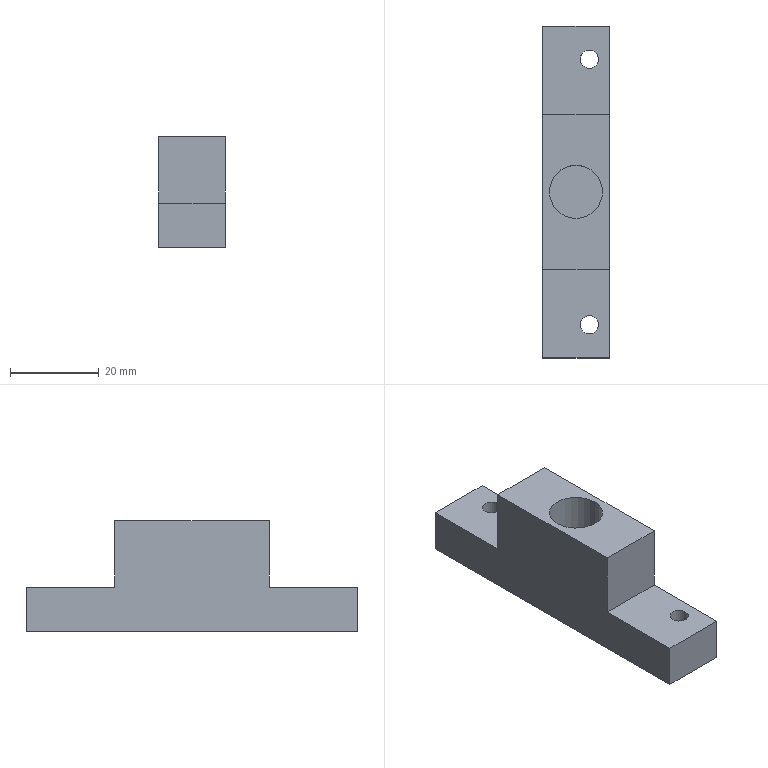Part | SolidWorks | features Cut 3, Extrusion 1 | 1 solid | 17 faces | box 15 x 75 x 25 mm | volume 16595 mm3 | plane 11 | cylinder 6 | commonest cylinder face diameters 4.134 x4 12 x2
STEP:
#1=CARTESIAN_POINT('',(-35.5,0.,5.));
#2=VERTEX_POINT('',#1);
#3=CARTESIAN_POINT('',(-23.5,0.,5.));
#4=VERTEX_POINT('',#3);
#5=CARTESIAN_POINT('',(-29.5,0.,5.));
#6=DIRECTION('',(0.,0.,1.));
#7=DIRECTION('',(1.,0.,0.));
#8=AXIS2_PLACEMENT_3D('',#5,#6,#7);
#9=CIRCLE('',#8,6.);
#10=EDGE_CURVE('',#2,#4,#9,.T.);
#11=ORIENTED_EDGE('',*,*,#10,.F.);
#12=CARTESIAN_POINT('',(-35.5,0.,25.));
#13=VERTEX_POINT('',#12);
#14=CARTESIAN_POINT('',(-35.5,0.,5.));
#15=DIRECTION('',(0.,0.,1.));
#16=VECTOR('',#15,1000.);
#17=LINE('',#14,#16);
#18=EDGE_CURVE('',#2,#13,#17,.T.);
#19=ORIENTED_EDGE('',*,*,#18,.T.);
#20=CARTESIAN_POINT('',(-23.5,0.,25.));
#21=VERTEX_POINT('',#20);
#22=CARTESIAN_POINT('',(-29.5,0.,25.));
#23=DIRECTION('',(0.,0.,1.));
#24=DIRECTION('',(1.,0.,0.));
#25=AXIS2_PLACEMENT_3D('',#22,#23,#24);
#26=CIRCLE('',#25,6.);
#27=EDGE_CURVE('',#13,#21,#26,.T.);
#28=ORIENTED_EDGE('',*,*,#27,.T.);
#29=CARTESIAN_POINT('',(-23.5,0.,5.));
#30=DIRECTION('',(0.,0.,1.));
#31=VECTOR('',#30,1000.);
#32=LINE('',#29,#31);
#33=EDGE_CURVE('',#4,#21,#32,.T.);
#34=ORIENTED_EDGE('',*,*,#33,.F.);
#35=EDGE_LOOP('',(#11,#19,#28,#34));
#36=FACE_OUTER_BOUND('',#35,.T.);
#37=CARTESIAN_POINT('',(-29.5,0.,5.));
#38=DIRECTION('',(0.,0.,1.));
#39=DIRECTION('',(1.,0.,0.));
#40=AXIS2_PLACEMENT_3D('',#37,#38,#39);
#41=CYLINDRICAL_SURFACE('',#40,6.);
#42=ADVANCED_FACE('',(#36),#41,.F.);
#43=CARTESIAN_POINT('',(-28.567,30.,0.));
#44=VERTEX_POINT('',#43);
#45=CARTESIAN_POINT('',(-24.433,30.,0.));
#46=VERTEX_POINT('',#45);
#47=CARTESIAN_POINT('',(-26.5,30.,0.));
#48=DIRECTION('',(0.,0.,1.));
#49=DIRECTION('',(1.,0.,0.));
#50=AXIS2_PLACEMENT_3D('',#47,#48,#49);
#51=CIRCLE('',#50,2.067);
#52=EDGE_CURVE('',#44,#46,#51,.T.);
#53=ORIENTED_EDGE('',*,*,#52,.F.);
#54=CARTESIAN_POINT('',(-28.567,30.,10.));
#55=VERTEX_POINT('',#54);
#56=CARTESIAN_POINT('',(-28.567,30.,0.));
#57=DIRECTION('',(0.,0.,1.));
#58=VECTOR('',#57,1000.);
#59=LINE('',#56,#58);
#60=EDGE_CURVE('',#44,#55,#59,.T.);
#61=ORIENTED_EDGE('',*,*,#60,.T.);
#62=CARTESIAN_POINT('',(-24.433,30.,10.));
#63=VERTEX_POINT('',#62);
#64=CARTESIAN_POINT('',(-26.5,30.,10.));
#65=DIRECTION('',(0.,0.,1.));
#66=DIRECTION('',(-1.,0.,0.));
#67=AXIS2_PLACEMENT_3D('',#64,#65,#66);
#68=CIRCLE('',#67,2.067);
#69=EDGE_CURVE('',#55,#63,#68,.T.);
#70=ORIENTED_EDGE('',*,*,#69,.T.);
#71=CARTESIAN_POINT('',(-24.433,30.,0.));
#72=DIRECTION('',(0.,0.,1.));
#73=VECTOR('',#72,1000.);
#74=LINE('',#71,#73);
#75=EDGE_CURVE('',#46,#63,#74,.T.);
#76=ORIENTED_EDGE('',*,*,#75,.F.);
#77=EDGE_LOOP('',(#53,#61,#70,#76));
#78=FACE_OUTER_BOUND('',#77,.T.);
#79=CARTESIAN_POINT('',(-26.5,30.,0.));
#80=DIRECTION('',(0.,0.,1.));
#81=DIRECTION('',(1.,0.,0.));
#82=AXIS2_PLACEMENT_3D('',#79,#80,#81);
#83=CYLINDRICAL_SURFACE('',#82,2.067);
#84=ADVANCED_FACE('',(#78),#83,.F.);
#85=CARTESIAN_POINT('',(-28.567,-30.,0.));
#86=VERTEX_POINT('',#85);
#87=CARTESIAN_POINT('',(-24.433,-30.,0.));
#88=VERTEX_POINT('',#87);
#89=CARTESIAN_POINT('',(-26.5,-30.,0.));
#90=DIRECTION('',(0.,0.,1.));
#91=DIRECTION('',(1.,0.,0.));
#92=AXIS2_PLACEMENT_3D('',#89,#90,#91);
#93=CIRCLE('',#92,2.067);
#94=EDGE_CURVE('',#86,#88,#93,.T.);
#95=ORIENTED_EDGE('',*,*,#94,.F.);
#96=CARTESIAN_POINT('',(-28.567,-30.,10.));
#97=VERTEX_POINT('',#96);
#98=CARTESIAN_POINT('',(-28.567,-30.,0.));
#99=DIRECTION('',(0.,0.,1.));
#100=VECTOR('',#99,1000.);
#101=LINE('',#98,#100);
#102=EDGE_CURVE('',#86,#97,#101,.T.);
#103=ORIENTED_EDGE('',*,*,#102,.T.);
#104=CARTESIAN_POINT('',(-24.433,-30.,10.));
#105=VERTEX_POINT('',#104);
#106=CARTESIAN_POINT('',(-26.5,-30.,10.));
#107=DIRECTION('',(0.,0.,-1.));
#108=DIRECTION('',(1.,0.,0.));
#109=AXIS2_PLACEMENT_3D('',#106,#107,#108);
#110=CIRCLE('',#109,2.067);
#111=EDGE_CURVE('',#105,#97,#110,.T.);
#112=ORIENTED_EDGE('',*,*,#111,.F.);
#113=CARTESIAN_POINT('',(-24.433,-30.,0.));
#114=DIRECTION('',(0.,0.,1.));
#115=VECTOR('',#114,1000.);
#116=LINE('',#113,#115);
#117=EDGE_CURVE('',#88,#105,#116,.T.);
#118=ORIENTED_EDGE('',*,*,#117,.F.);
#119=EDGE_LOOP('',(#95,#103,#112,#118));
#120=FACE_OUTER_BOUND('',#119,.T.);
#121=CARTESIAN_POINT('',(-26.5,-30.,0.));
#122=DIRECTION('',(0.,0.,1.));
#123=DIRECTION('',(1.,0.,0.));
#124=AXIS2_PLACEMENT_3D('',#121,#122,#123);
#125=CYLINDRICAL_SURFACE('',#124,2.067);
#126=ADVANCED_FACE('',(#120),#125,.F.);
#127=CARTESIAN_POINT('',(-37.,-37.5,10.));
#128=VERTEX_POINT('',#127);
#129=CARTESIAN_POINT('',(-22.,-37.5,10.));
#130=VERTEX_POINT('',#129);
#131=CARTESIAN_POINT('',(-37.,-37.5,10.));
#132=DIRECTION('',(1.,0.,0.));
#133=VECTOR('',#132,1000.);
#134=LINE('',#131,#133);
#135=EDGE_CURVE('',#128,#130,#134,.T.);
#136=ORIENTED_EDGE('',*,*,#135,.F.);
#137=CARTESIAN_POINT('',(-37.,-37.5,0.));
#138=VERTEX_POINT('',#137);
#139=CARTESIAN_POINT('',(-37.,-37.5,25.));
#140=DIRECTION('',(0.,0.,-1.));
#141=VECTOR('',#140,1000.);
#142=LINE('',#139,#141);
#143=EDGE_CURVE('',#128,#138,#142,.T.);
#144=ORIENTED_EDGE('',*,*,#143,.T.);
#145=CARTESIAN_POINT('',(-22.,-37.5,0.));
#146=VERTEX_POINT('',#145);
#147=CARTESIAN_POINT('',(-22.,-37.5,0.));
#148=DIRECTION('',(1.,0.,0.));
#149=VECTOR('',#148,1000.);
#150=LINE('',#147,#149);
#151=EDGE_CURVE('',#138,#146,#150,.T.);
#152=ORIENTED_EDGE('',*,*,#151,.T.);
#153=CARTESIAN_POINT('',(-22.,-37.5,25.));
#154=DIRECTION('',(0.,0.,-1.));
#155=VECTOR('',#154,1000.);
#156=LINE('',#153,#155);
#157=EDGE_CURVE('',#130,#146,#156,.T.);
#158=ORIENTED_EDGE('',*,*,#157,.F.);
#159=EDGE_LOOP('',(#136,#144,#152,#158));
#160=FACE_OUTER_BOUND('',#159,.T.);
#161=CARTESIAN_POINT('',(-22.,-37.5,25.));
#162=DIRECTION('',(0.,1.,0.));
#163=DIRECTION('',(0.,0.,1.));
#164=AXIS2_PLACEMENT_3D('',#161,#162,#163);
#165=PLANE('',#164);
#166=ADVANCED_FACE('',(#160),#165,.F.);
#167=ORIENTED_EDGE('',*,*,#102,.F.);
#168=CARTESIAN_POINT('',(-26.5,-30.,0.));
#169=DIRECTION('',(0.,0.,1.));
#170=DIRECTION('',(1.,0.,0.));
#171=AXIS2_PLACEMENT_3D('',#168,#169,#170);
#172=CIRCLE('',#171,2.067);
#173=EDGE_CURVE('',#88,#86,#172,.T.);
#174=ORIENTED_EDGE('',*,*,#173,.F.);
#175=ORIENTED_EDGE('',*,*,#117,.T.);
#176=CARTESIAN_POINT('',(-26.5,-30.,10.));
#177=DIRECTION('',(0.,0.,-1.));
#178=DIRECTION('',(1.,0.,0.));
#179=AXIS2_PLACEMENT_3D('',#176,#177,#178);
#180=CIRCLE('',#179,2.067);
#181=EDGE_CURVE('',#97,#105,#180,.T.);
#182=ORIENTED_EDGE('',*,*,#181,.F.);
#183=EDGE_LOOP('',(#167,#174,#175,#182));
#184=FACE_OUTER_BOUND('',#183,.T.);
#185=CARTESIAN_POINT('',(-26.5,-30.,0.));
#186=DIRECTION('',(0.,0.,1.));
#187=DIRECTION('',(1.,0.,0.));
#188=AXIS2_PLACEMENT_3D('',#185,#186,#187);
#189=CYLINDRICAL_SURFACE('',#188,2.067);
#190=ADVANCED_FACE('',(#184),#189,.F.);
#191=CARTESIAN_POINT('',(-37.,37.5,10.));
#192=VERTEX_POINT('',#191);
#193=CARTESIAN_POINT('',(-37.,37.5,0.));
#194=VERTEX_POINT('',#193);
#195=CARTESIAN_POINT('',(-37.,37.5,25.));
#196=DIRECTION('',(0.,0.,-1.));
#197=VECTOR('',#196,1000.);
#198=LINE('',#195,#197);
#199=EDGE_CURVE('',#192,#194,#198,.T.);
#200=ORIENTED_EDGE('',*,*,#199,.F.);
#201=CARTESIAN_POINT('',(-22.,37.5,10.));
#202=VERTEX_POINT('',#201);
#203=CARTESIAN_POINT('',(-37.,37.5,10.));
#204=DIRECTION('',(-1.,0.,0.));
#205=VECTOR('',#204,1000.);
#206=LINE('',#203,#205);
#207=EDGE_CURVE('',#202,#192,#206,.T.);
#208=ORIENTED_EDGE('',*,*,#207,.F.);
#209=CARTESIAN_POINT('',(-22.,37.5,0.));
#210=VERTEX_POINT('',#209);
#211=CARTESIAN_POINT('',(-22.,37.5,25.));
#212=DIRECTION('',(0.,0.,-1.));
#213=VECTOR('',#212,1000.);
#214=LINE('',#211,#213);
#215=EDGE_CURVE('',#202,#210,#214,.T.);
#216=ORIENTED_EDGE('',*,*,#215,.T.);
#217=CARTESIAN_POINT('',(-37.,37.5,0.));
#218=DIRECTION('',(-1.,0.,0.));
#219=VECTOR('',#218,1000.);
#220=LINE('',#217,#219);
#221=EDGE_CURVE('',#210,#194,#220,.T.);
#222=ORIENTED_EDGE('',*,*,#221,.T.);
#223=EDGE_LOOP('',(#200,#208,#216,#222));
#224=FACE_OUTER_BOUND('',#223,.T.);
#225=CARTESIAN_POINT('',(-37.,37.5,25.));
#226=DIRECTION('',(0.,-1.,0.));
#227=DIRECTION('',(0.,0.,-1.));
#228=AXIS2_PLACEMENT_3D('',#225,#226,#227);
#229=PLANE('',#228);
#230=ADVANCED_FACE('',(#224),#229,.F.);
#231=CARTESIAN_POINT('',(-37.,17.5,25.));
#232=VERTEX_POINT('',#231);
#233=CARTESIAN_POINT('',(-37.,-17.5,25.));
#234=VERTEX_POINT('',#233);
#235=CARTESIAN_POINT('',(-37.,-37.5,25.));
#236=DIRECTION('',(0.,-1.,0.));
#237=VECTOR('',#236,1000.);
#238=LINE('',#235,#237);
#239=EDGE_CURVE('',#232,#234,#238,.T.);
#240=ORIENTED_EDGE('',*,*,#239,.F.);
#241=CARTESIAN_POINT('',(-37.,17.5,10.));
#242=VERTEX_POINT('',#241);
#243=CARTESIAN_POINT('',(-37.,17.5,10.));
#244=DIRECTION('',(0.,0.,1.));
#245=VECTOR('',#244,1000.);
#246=LINE('',#243,#245);
#247=EDGE_CURVE('',#242,#232,#246,.T.);
#248=ORIENTED_EDGE('',*,*,#247,.F.);
#249=CARTESIAN_POINT('',(-37.,17.5,10.));
#250=DIRECTION('',(0.,-1.,0.));
#251=VECTOR('',#250,1000.);
#252=LINE('',#249,#251);
#253=EDGE_CURVE('',#192,#242,#252,.T.);
#254=ORIENTED_EDGE('',*,*,#253,.F.);
#255=ORIENTED_EDGE('',*,*,#199,.T.);
#256=CARTESIAN_POINT('',(-37.,-37.5,0.));
#257=DIRECTION('',(0.,-1.,0.));
#258=VECTOR('',#257,1000.);
#259=LINE('',#256,#258);
#260=EDGE_CURVE('',#194,#138,#259,.T.);
#261=ORIENTED_EDGE('',*,*,#260,.T.);
#262=ORIENTED_EDGE('',*,*,#143,.F.);
#263=CARTESIAN_POINT('',(-37.,-17.5,10.));
#264=VERTEX_POINT('',#263);
#265=CARTESIAN_POINT('',(-37.,-17.5,10.));
#266=DIRECTION('',(0.,-1.,0.));
#267=VECTOR('',#266,1000.);
#268=LINE('',#265,#267);
#269=EDGE_CURVE('',#264,#128,#268,.T.);
#270=ORIENTED_EDGE('',*,*,#269,.F.);
#271=CARTESIAN_POINT('',(-37.,-17.5,10.));
#272=DIRECTION('',(0.,0.,1.));
#273=VECTOR('',#272,1000.);
#274=LINE('',#271,#273);
#275=EDGE_CURVE('',#264,#234,#274,.T.);
#276=ORIENTED_EDGE('',*,*,#275,.T.);
#277=EDGE_LOOP('',(#240,#248,#254,#255,#261,#262,#270,#276));
#278=FACE_OUTER_BOUND('',#277,.T.);
#279=CARTESIAN_POINT('',(-37.,-37.5,25.));
#280=DIRECTION('',(1.,0.,0.));
#281=DIRECTION('',(0.,0.,-1.));
#282=AXIS2_PLACEMENT_3D('',#279,#280,#281);
#283=PLANE('',#282);
#284=ADVANCED_FACE('',(#278),#283,.F.);
#285=CARTESIAN_POINT('',(-22.,17.5,10.));
#286=VERTEX_POINT('',#285);
#287=CARTESIAN_POINT('',(-22.,37.5,10.));
#288=DIRECTION('',(0.,1.,0.));
#289=VECTOR('',#288,1000.);
#290=LINE('',#287,#289);
#291=EDGE_CURVE('',#286,#202,#290,.T.);
#292=ORIENTED_EDGE('',*,*,#291,.F.);
#293=CARTESIAN_POINT('',(-22.,17.5,25.));
#294=VERTEX_POINT('',#293);
#295=CARTESIAN_POINT('',(-22.,17.5,10.));
#296=DIRECTION('',(0.,0.,1.));
#297=VECTOR('',#296,1000.);
#298=LINE('',#295,#297);
#299=EDGE_CURVE('',#286,#294,#298,.T.);
#300=ORIENTED_EDGE('',*,*,#299,.T.);
#301=CARTESIAN_POINT('',(-22.,-17.5,25.));
#302=VERTEX_POINT('',#301);
#303=CARTESIAN_POINT('',(-22.,37.5,25.));
#304=DIRECTION('',(0.,1.,0.));
#305=VECTOR('',#304,1000.);
#306=LINE('',#303,#305);
#307=EDGE_CURVE('',#302,#294,#306,.T.);
#308=ORIENTED_EDGE('',*,*,#307,.F.);
#309=CARTESIAN_POINT('',(-22.,-17.5,10.));
#310=VERTEX_POINT('',#309);
#311=CARTESIAN_POINT('',(-22.,-17.5,10.));
#312=DIRECTION('',(0.,0.,1.));
#313=VECTOR('',#312,1000.);
#314=LINE('',#311,#313);
#315=EDGE_CURVE('',#310,#302,#314,.T.);
#316=ORIENTED_EDGE('',*,*,#315,.F.);
#317=CARTESIAN_POINT('',(-22.,-37.5,10.));
#318=DIRECTION('',(0.,1.,0.));
#319=VECTOR('',#318,1000.);
#320=LINE('',#317,#319);
#321=EDGE_CURVE('',#130,#310,#320,.T.);
#322=ORIENTED_EDGE('',*,*,#321,.F.);
#323=ORIENTED_EDGE('',*,*,#157,.T.);
#324=CARTESIAN_POINT('',(-22.,37.5,0.));
#325=DIRECTION('',(0.,1.,0.));
#326=VECTOR('',#325,1000.);
#327=LINE('',#324,#326);
#328=EDGE_CURVE('',#146,#210,#327,.T.);
#329=ORIENTED_EDGE('',*,*,#328,.T.);
#330=ORIENTED_EDGE('',*,*,#215,.F.);
#331=EDGE_LOOP('',(#292,#300,#308,#316,#322,#323,#329,#330));
#332=FACE_OUTER_BOUND('',#331,.T.);
#333=CARTESIAN_POINT('',(-22.,37.5,25.));
#334=DIRECTION('',(-1.,0.,0.));
#335=DIRECTION('',(0.,-1.,0.));
#336=AXIS2_PLACEMENT_3D('',#333,#334,#335);
#337=PLANE('',#336);
#338=ADVANCED_FACE('',(#332),#337,.F.);
#339=CARTESIAN_POINT('',(-29.5,0.,25.));
#340=DIRECTION('',(0.,0.,1.));
#341=DIRECTION('',(1.,0.,0.));
#342=AXIS2_PLACEMENT_3D('',#339,#340,#341);
#343=CIRCLE('',#342,6.);
#344=EDGE_CURVE('',#21,#13,#343,.T.);
#345=ORIENTED_EDGE('',*,*,#344,.F.);
#346=ORIENTED_EDGE('',*,*,#27,.F.);
#347=EDGE_LOOP('',(#345,#346));
#348=FACE_BOUND('',#347,.T.);
#349=ORIENTED_EDGE('',*,*,#307,.T.);
#350=CARTESIAN_POINT('',(-22.,17.5,25.));
#351=DIRECTION('',(1.,0.,0.));
#352=VECTOR('',#351,1000.);
#353=LINE('',#350,#352);
#354=EDGE_CURVE('',#232,#294,#353,.T.);
#355=ORIENTED_EDGE('',*,*,#354,.F.);
#356=ORIENTED_EDGE('',*,*,#239,.T.);
#357=CARTESIAN_POINT('',(-22.,-17.5,25.));
#358=DIRECTION('',(-1.,0.,0.));
#359=VECTOR('',#358,1000.);
#360=LINE('',#357,#359);
#361=EDGE_CURVE('',#302,#234,#360,.T.);
#362=ORIENTED_EDGE('',*,*,#361,.F.);
#363=EDGE_LOOP('',(#349,#355,#356,#362));
#364=FACE_OUTER_BOUND('',#363,.T.);
#365=CARTESIAN_POINT('',(0.,0.,25.));
#366=DIRECTION('',(0.,0.,-1.));
#367=DIRECTION('',(-1.,0.,0.));
#368=AXIS2_PLACEMENT_3D('',#365,#366,#367);
#369=PLANE('',#368);
#370=ADVANCED_FACE('',(#348,#364),#369,.F.);
#371=CARTESIAN_POINT('',(-26.5,30.,0.));
#372=DIRECTION('',(0.,0.,1.));
#373=DIRECTION('',(1.,0.,0.));
#374=AXIS2_PLACEMENT_3D('',#371,#372,#373);
#375=CIRCLE('',#374,2.067);
#376=EDGE_CURVE('',#46,#44,#375,.T.);
#377=ORIENTED_EDGE('',*,*,#376,.T.);
#378=ORIENTED_EDGE('',*,*,#52,.T.);
#379=EDGE_LOOP('',(#377,#378));
#380=FACE_BOUND('',#379,.T.);
#381=ORIENTED_EDGE('',*,*,#173,.T.);
#382=ORIENTED_EDGE('',*,*,#94,.T.);
#383=EDGE_LOOP('',(#381,#382));
#384=FACE_BOUND('',#383,.T.);
#385=ORIENTED_EDGE('',*,*,#221,.F.);
#386=ORIENTED_EDGE('',*,*,#328,.F.);
#387=ORIENTED_EDGE('',*,*,#151,.F.);
#388=ORIENTED_EDGE('',*,*,#260,.F.);
#389=EDGE_LOOP('',(#385,#386,#387,#388));
#390=FACE_OUTER_BOUND('',#389,.T.);
#391=CARTESIAN_POINT('',(0.,0.,0.));
#392=DIRECTION('',(0.,0.,-1.));
#393=DIRECTION('',(-1.,0.,0.));
#394=AXIS2_PLACEMENT_3D('',#391,#392,#393);
#395=PLANE('',#394);
#396=ADVANCED_FACE('',(#380,#384,#390),#395,.T.);
#397=ORIENTED_EDGE('',*,*,#60,.F.);
#398=ORIENTED_EDGE('',*,*,#376,.F.);
#399=ORIENTED_EDGE('',*,*,#75,.T.);
#400=CARTESIAN_POINT('',(-26.5,30.,10.));
#401=DIRECTION('',(0.,0.,1.));
#402=DIRECTION('',(-1.,0.,0.));
#403=AXIS2_PLACEMENT_3D('',#400,#401,#402);
#404=CIRCLE('',#403,2.067);
#405=EDGE_CURVE('',#63,#55,#404,.T.);
#406=ORIENTED_EDGE('',*,*,#405,.T.);
#407=EDGE_LOOP('',(#397,#398,#399,#406));
#408=FACE_OUTER_BOUND('',#407,.T.);
#409=CARTESIAN_POINT('',(-26.5,30.,0.));
#410=DIRECTION('',(0.,0.,1.));
#411=DIRECTION('',(1.,0.,0.));
#412=AXIS2_PLACEMENT_3D('',#409,#410,#411);
#413=CYLINDRICAL_SURFACE('',#412,2.067);
#414=ADVANCED_FACE('',(#408),#413,.F.);
#415=ORIENTED_EDGE('',*,*,#253,.T.);
#416=CARTESIAN_POINT('',(-22.,17.5,10.));
#417=DIRECTION('',(1.,0.,0.));
#418=VECTOR('',#417,1000.);
#419=LINE('',#416,#418);
#420=EDGE_CURVE('',#242,#286,#419,.T.);
#421=ORIENTED_EDGE('',*,*,#420,.T.);
#422=ORIENTED_EDGE('',*,*,#291,.T.);
#423=ORIENTED_EDGE('',*,*,#207,.T.);
#424=EDGE_LOOP('',(#415,#421,#422,#423));
#425=FACE_OUTER_BOUND('',#424,.T.);
#426=ORIENTED_EDGE('',*,*,#405,.F.);
#427=ORIENTED_EDGE('',*,*,#69,.F.);
#428=EDGE_LOOP('',(#426,#427));
#429=FACE_BOUND('',#428,.T.);
#430=CARTESIAN_POINT('',(0.,0.,10.));
#431=DIRECTION('',(0.,0.,-1.));
#432=DIRECTION('',(-1.,0.,0.));
#433=AXIS2_PLACEMENT_3D('',#430,#431,#432);
#434=PLANE('',#433);
#435=ADVANCED_FACE('',(#425,#429),#434,.F.);
#436=ORIENTED_EDGE('',*,*,#354,.T.);
#437=ORIENTED_EDGE('',*,*,#299,.F.);
#438=ORIENTED_EDGE('',*,*,#420,.F.);
#439=ORIENTED_EDGE('',*,*,#247,.T.);
#440=EDGE_LOOP('',(#436,#437,#438,#439));
#441=FACE_OUTER_BOUND('',#440,.T.);
#442=CARTESIAN_POINT('',(-22.,17.5,10.));
#443=DIRECTION('',(0.,-1.,0.));
#444=DIRECTION('',(0.,0.,-1.));
#445=AXIS2_PLACEMENT_3D('',#442,#443,#444);
#446=PLANE('',#445);
#447=ADVANCED_FACE('',(#441),#446,.F.);
#448=ORIENTED_EDGE('',*,*,#321,.T.);
#449=CARTESIAN_POINT('',(-22.,-17.5,10.));
#450=DIRECTION('',(-1.,0.,0.));
#451=VECTOR('',#450,1000.);
#452=LINE('',#449,#451);
#453=EDGE_CURVE('',#310,#264,#452,.T.);
#454=ORIENTED_EDGE('',*,*,#453,.T.);
#455=ORIENTED_EDGE('',*,*,#269,.T.);
#456=ORIENTED_EDGE('',*,*,#135,.T.);
#457=EDGE_LOOP('',(#448,#454,#455,#456));
#458=FACE_OUTER_BOUND('',#457,.T.);
#459=ORIENTED_EDGE('',*,*,#111,.T.);
#460=ORIENTED_EDGE('',*,*,#181,.T.);
#461=EDGE_LOOP('',(#459,#460));
#462=FACE_BOUND('',#461,.T.);
#463=CARTESIAN_POINT('',(0.,0.,10.));
#464=DIRECTION('',(0.,0.,1.));
#465=DIRECTION('',(1.,0.,0.));
#466=AXIS2_PLACEMENT_3D('',#463,#464,#465);
#467=PLANE('',#466);
#468=ADVANCED_FACE('',(#458,#462),#467,.T.);
#469=ORIENTED_EDGE('',*,*,#361,.T.);
#470=ORIENTED_EDGE('',*,*,#275,.F.);
#471=ORIENTED_EDGE('',*,*,#453,.F.);
#472=ORIENTED_EDGE('',*,*,#315,.T.);
#473=EDGE_LOOP('',(#469,#470,#471,#472));
#474=FACE_OUTER_BOUND('',#473,.T.);
#475=CARTESIAN_POINT('',(-22.,-17.5,10.));
#476=DIRECTION('',(0.,1.,0.));
#477=DIRECTION('',(0.,0.,1.));
#478=AXIS2_PLACEMENT_3D('',#475,#476,#477);
#479=PLANE('',#478);
#480=ADVANCED_FACE('',(#474),#479,.F.);
#481=ORIENTED_EDGE('',*,*,#18,.F.);
#482=CARTESIAN_POINT('',(-29.5,0.,5.));
#483=DIRECTION('',(0.,0.,1.));
#484=DIRECTION('',(1.,0.,0.));
#485=AXIS2_PLACEMENT_3D('',#482,#483,#484);
#486=CIRCLE('',#485,6.);
#487=EDGE_CURVE('',#4,#2,#486,.T.);
#488=ORIENTED_EDGE('',*,*,#487,.F.);
#489=ORIENTED_EDGE('',*,*,#33,.T.);
#490=ORIENTED_EDGE('',*,*,#344,.T.);
#491=EDGE_LOOP('',(#481,#488,#489,#490));
#492=FACE_OUTER_BOUND('',#491,.T.);
#493=CARTESIAN_POINT('',(-29.5,0.,5.));
#494=DIRECTION('',(0.,0.,1.));
#495=DIRECTION('',(1.,0.,0.));
#496=AXIS2_PLACEMENT_3D('',#493,#494,#495);
#497=CYLINDRICAL_SURFACE('',#496,6.);
#498=ADVANCED_FACE('',(#492),#497,.F.);
#499=ORIENTED_EDGE('',*,*,#487,.T.);
#500=ORIENTED_EDGE('',*,*,#10,.T.);
#501=EDGE_LOOP('',(#499,#500));
#502=FACE_OUTER_BOUND('',#501,.T.);
#503=CARTESIAN_POINT('',(-29.5,0.,5.));
#504=DIRECTION('',(0.,0.,1.));
#505=DIRECTION('',(1.,0.,0.));
#506=AXIS2_PLACEMENT_3D('',#503,#504,#505);
#507=PLANE('',#506);
#508=ADVANCED_FACE('',(#502),#507,.T.);
#509=CLOSED_SHELL('',(#42,#84,#126,#166,#190,#230,#284,#338,#370,#396,#414,#435,#447,#468,#480,#498,#508));
#510=MANIFOLD_SOLID_BREP('',#509);
#511=CARTESIAN_POINT('',(0.,0.,0.));
#512=DIRECTION('',(0.,0.,1.));
#513=DIRECTION('',(1.,0.,0.));
#514=AXIS2_PLACEMENT_3D('',#511,#512,#513);
#515=(LENGTH_UNIT()NAMED_UNIT(*)SI_UNIT(.MILLI.,.METRE.));
#516=UNCERTAINTY_MEASURE_WITH_UNIT(LENGTH_MEASURE(0.00001),#515,'','');
#517=(NAMED_UNIT(*)PLANE_ANGLE_UNIT()SI_UNIT($,.RADIAN.));
#518=(NAMED_UNIT(*)SI_UNIT($,.STERADIAN.)SOLID_ANGLE_UNIT());
#519=(GEOMETRIC_REPRESENTATION_CONTEXT(3)GLOBAL_UNCERTAINTY_ASSIGNED_CONTEXT((#516))GLOBAL_UNIT_ASSIGNED_CONTEXT((#515,#517,#518))REPRESENTATION_CONTEXT('',''));
#520=ADVANCED_BREP_SHAPE_REPRESENTATION('',(#510,#514),#519);